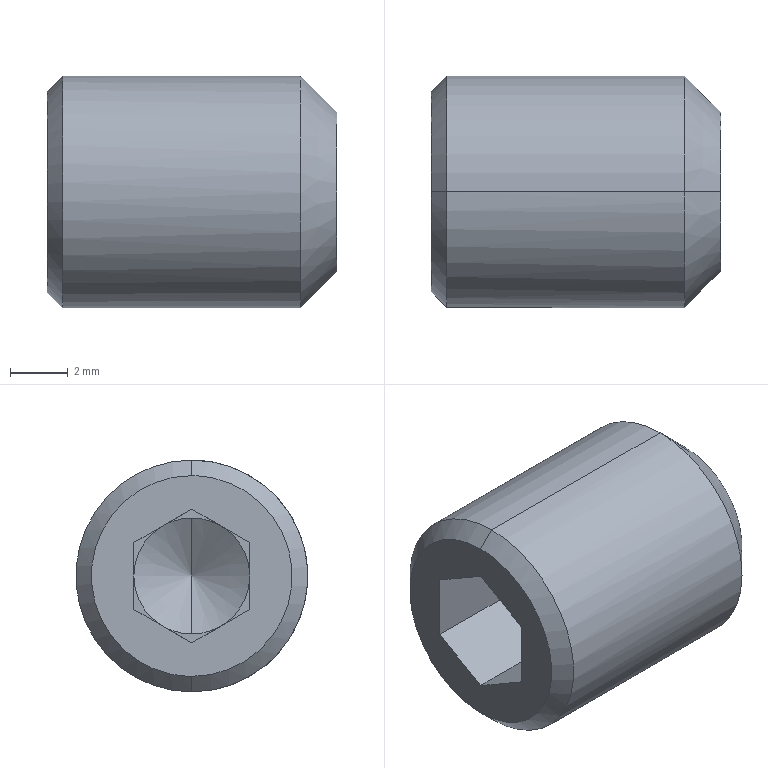Part | STEP file | 103000006174_M8×10 | 1 solid | 22 faces | box 10 x 8 x 8 mm | volume 407.497 mm3 | plane 14 | cone 6 | cylinder 2 | commonest cylinder face diameters 8 x2
STEP:
#1=CARTESIAN_POINT('',(6.155,0.,0.));
#2=VERTEX_POINT('',#1);
#3=CARTESIAN_POINT('',(5.,0.,2.));
#4=VERTEX_POINT('',#3);
#5=CARTESIAN_POINT('',(-250493.845,0.,433878.727));
#6=DIRECTION('',(-0.5,0.,0.866));
#7=VECTOR('',#6,1.);
#8=LINE('',#5,#7);
#9=EDGE_CURVE('',#2,#4,#8,.T.);
#10=ORIENTED_EDGE('',*,*,#9,.F.);
#11=CARTESIAN_POINT('',(5.,0.,-2.));
#12=VERTEX_POINT('',#11);
#13=CARTESIAN_POINT('',(-250493.845,0.,-433878.727));
#14=DIRECTION('',(-0.5,0.,-0.866));
#15=VECTOR('',#14,1.);
#16=LINE('',#13,#15);
#17=EDGE_CURVE('',#2,#12,#16,.T.);
#18=ORIENTED_EDGE('',*,*,#17,.T.);
#19=CARTESIAN_POINT('',(5.,-1.,-1.732));
#20=VERTEX_POINT('',#19);
#21=CARTESIAN_POINT('',(5.,0.,0.));
#22=DIRECTION('',(-1.,0.,0.));
#23=AXIS2_PLACEMENT_3D('',#21,#22,$);
#24=CIRCLE('',#23,2.);
#25=EDGE_CURVE('',#12,#20,#24,.T.);
#26=ORIENTED_EDGE('',*,*,#25,.T.);
#27=CARTESIAN_POINT('',(5.,-2.,0.));
#28=VERTEX_POINT('',#27);
#29=CARTESIAN_POINT('',(5.,0.,0.));
#30=DIRECTION('',(-1.,0.,0.));
#31=AXIS2_PLACEMENT_3D('',#29,#30,$);
#32=CIRCLE('',#31,2.);
#33=EDGE_CURVE('',#20,#28,#32,.T.);
#34=ORIENTED_EDGE('',*,*,#33,.T.);
#35=CARTESIAN_POINT('',(5.,-1.,1.732));
#36=VERTEX_POINT('',#35);
#37=CARTESIAN_POINT('',(5.,0.,0.));
#38=DIRECTION('',(-1.,0.,0.));
#39=AXIS2_PLACEMENT_3D('',#37,#38,$);
#40=CIRCLE('',#39,2.);
#41=EDGE_CURVE('',#28,#36,#40,.T.);
#42=ORIENTED_EDGE('',*,*,#41,.T.);
#43=CARTESIAN_POINT('',(5.,0.,0.));
#44=DIRECTION('',(-1.,0.,0.));
#45=AXIS2_PLACEMENT_3D('',#43,#44,$);
#46=CIRCLE('',#45,2.);
#47=EDGE_CURVE('',#36,#4,#46,.T.);
#48=ORIENTED_EDGE('',*,*,#47,.T.);
#49=EDGE_LOOP('',(#10,#18,#26,#34,#42,#48));
#50=FACE_OUTER_BOUND('',#49,.T.);
#51=CARTESIAN_POINT('',(-993.845,0.,0.));
#52=DIRECTION('',(-1.,0.,0.));
#53=DIRECTION('',(0.,0.,-1.));
#54=AXIS2_PLACEMENT_3D('',#51,#52,#53);
#55=CONICAL_SURFACE('',#54,1732.051,1.047);
#56=ADVANCED_FACE('',(#50),#55,.F.);
#57=ORIENTED_EDGE('',*,*,#17,.F.);
#58=ORIENTED_EDGE('',*,*,#9,.T.);
#59=CARTESIAN_POINT('',(5.,1.,1.732));
#60=VERTEX_POINT('',#59);
#61=CARTESIAN_POINT('',(5.,0.,0.));
#62=DIRECTION('',(-1.,0.,0.));
#63=AXIS2_PLACEMENT_3D('',#61,#62,$);
#64=CIRCLE('',#63,2.);
#65=EDGE_CURVE('',#4,#60,#64,.T.);
#66=ORIENTED_EDGE('',*,*,#65,.T.);
#67=CARTESIAN_POINT('',(5.,2.,0.));
#68=VERTEX_POINT('',#67);
#69=CARTESIAN_POINT('',(5.,0.,0.));
#70=DIRECTION('',(-1.,0.,0.));
#71=AXIS2_PLACEMENT_3D('',#69,#70,$);
#72=CIRCLE('',#71,2.);
#73=EDGE_CURVE('',#60,#68,#72,.T.);
#74=ORIENTED_EDGE('',*,*,#73,.T.);
#75=CARTESIAN_POINT('',(5.,1.,-1.732));
#76=VERTEX_POINT('',#75);
#77=CARTESIAN_POINT('',(5.,0.,0.));
#78=DIRECTION('',(-1.,0.,0.));
#79=AXIS2_PLACEMENT_3D('',#77,#78,$);
#80=CIRCLE('',#79,2.);
#81=EDGE_CURVE('',#68,#76,#80,.T.);
#82=ORIENTED_EDGE('',*,*,#81,.T.);
#83=CARTESIAN_POINT('',(5.,0.,0.));
#84=DIRECTION('',(-1.,0.,0.));
#85=AXIS2_PLACEMENT_3D('',#83,#84,$);
#86=CIRCLE('',#85,2.);
#87=EDGE_CURVE('',#76,#12,#86,.T.);
#88=ORIENTED_EDGE('',*,*,#87,.T.);
#89=EDGE_LOOP('',(#57,#58,#66,#74,#82,#88));
#90=FACE_OUTER_BOUND('',#89,.T.);
#91=CARTESIAN_POINT('',(-993.845,0.,0.));
#92=DIRECTION('',(-1.,0.,0.));
#93=DIRECTION('',(0.,0.,1.));
#94=AXIS2_PLACEMENT_3D('',#91,#92,#93);
#95=CONICAL_SURFACE('',#94,1732.051,1.047);
#96=ADVANCED_FACE('',(#90),#95,.F.);
#97=ORIENTED_EDGE('',*,*,#87,.F.);
#98=CARTESIAN_POINT('',(5.,0.,-2.309));
#99=VERTEX_POINT('',#98);
#100=CARTESIAN_POINT('',(5.,0.5,-2.021));
#101=DIRECTION('',(0.,-0.866,-0.5));
#102=VECTOR('',#101,1.);
#103=LINE('',#100,#102);
#104=EDGE_CURVE('',#76,#99,#103,.T.);
#105=ORIENTED_EDGE('',*,*,#104,.T.);
#106=CARTESIAN_POINT('',(5.,-0.5,-2.021));
#107=DIRECTION('',(0.,-0.866,0.5));
#108=VECTOR('',#107,1.);
#109=LINE('',#106,#108);
#110=EDGE_CURVE('',#99,#20,#109,.T.);
#111=ORIENTED_EDGE('',*,*,#110,.T.);
#112=ORIENTED_EDGE('',*,*,#25,.F.);
#113=EDGE_LOOP('',(#97,#105,#111,#112));
#114=FACE_OUTER_BOUND('',#113,.T.);
#115=CARTESIAN_POINT('',(5.,0.,-2.309));
#116=DIRECTION('',(1.,0.,0.));
#117=DIRECTION('',(0.,0.,-1.));
#118=AXIS2_PLACEMENT_3D('',#115,#116,#117);
#119=PLANE('',#118);
#120=ADVANCED_FACE('',(#114),#119,.F.);
#121=ORIENTED_EDGE('',*,*,#33,.F.);
#122=CARTESIAN_POINT('',(5.,-2.,-1.155));
#123=VERTEX_POINT('',#122);
#124=CARTESIAN_POINT('',(5.,-1.5,-1.443));
#125=DIRECTION('',(0.,-0.866,0.5));
#126=VECTOR('',#125,1.);
#127=LINE('',#124,#126);
#128=EDGE_CURVE('',#20,#123,#127,.T.);
#129=ORIENTED_EDGE('',*,*,#128,.T.);
#130=CARTESIAN_POINT('',(5.,-2.,-0.5774));
#131=DIRECTION('',(0.,0.,1.));
#132=VECTOR('',#131,1.);
#133=LINE('',#130,#132);
#134=EDGE_CURVE('',#123,#28,#133,.T.);
#135=ORIENTED_EDGE('',*,*,#134,.T.);
#136=EDGE_LOOP('',(#121,#129,#135));
#137=FACE_OUTER_BOUND('',#136,.T.);
#138=CARTESIAN_POINT('',(5.,0.,-2.309));
#139=DIRECTION('',(1.,0.,0.));
#140=DIRECTION('',(0.,0.,-1.));
#141=AXIS2_PLACEMENT_3D('',#138,#139,#140);
#142=PLANE('',#141);
#143=ADVANCED_FACE('',(#137),#142,.F.);
#144=ORIENTED_EDGE('',*,*,#41,.F.);
#145=CARTESIAN_POINT('',(5.,-2.,1.155));
#146=VERTEX_POINT('',#145);
#147=CARTESIAN_POINT('',(5.,-2.,0.5774));
#148=DIRECTION('',(0.,0.,1.));
#149=VECTOR('',#148,1.);
#150=LINE('',#147,#149);
#151=EDGE_CURVE('',#28,#146,#150,.T.);
#152=ORIENTED_EDGE('',*,*,#151,.T.);
#153=CARTESIAN_POINT('',(5.,-1.5,1.443));
#154=DIRECTION('',(0.,0.866,0.5));
#155=VECTOR('',#154,1.);
#156=LINE('',#153,#155);
#157=EDGE_CURVE('',#146,#36,#156,.T.);
#158=ORIENTED_EDGE('',*,*,#157,.T.);
#159=EDGE_LOOP('',(#144,#152,#158));
#160=FACE_OUTER_BOUND('',#159,.T.);
#161=CARTESIAN_POINT('',(5.,0.,-2.309));
#162=DIRECTION('',(1.,0.,0.));
#163=DIRECTION('',(0.,0.,-1.));
#164=AXIS2_PLACEMENT_3D('',#161,#162,#163);
#165=PLANE('',#164);
#166=ADVANCED_FACE('',(#160),#165,.F.);
#167=ORIENTED_EDGE('',*,*,#47,.F.);
#168=CARTESIAN_POINT('',(5.,0.,2.309));
#169=VERTEX_POINT('',#168);
#170=CARTESIAN_POINT('',(5.,-0.5,2.021));
#171=DIRECTION('',(0.,0.866,0.5));
#172=VECTOR('',#171,1.);
#173=LINE('',#170,#172);
#174=EDGE_CURVE('',#36,#169,#173,.T.);
#175=ORIENTED_EDGE('',*,*,#174,.T.);
#176=CARTESIAN_POINT('',(5.,0.5,2.021));
#177=DIRECTION('',(0.,0.866,-0.5));
#178=VECTOR('',#177,1.);
#179=LINE('',#176,#178);
#180=EDGE_CURVE('',#169,#60,#179,.T.);
#181=ORIENTED_EDGE('',*,*,#180,.T.);
#182=ORIENTED_EDGE('',*,*,#65,.F.);
#183=EDGE_LOOP('',(#167,#175,#181,#182));
#184=FACE_OUTER_BOUND('',#183,.T.);
#185=CARTESIAN_POINT('',(5.,0.,-2.309));
#186=DIRECTION('',(1.,0.,0.));
#187=DIRECTION('',(0.,0.,-1.));
#188=AXIS2_PLACEMENT_3D('',#185,#186,#187);
#189=PLANE('',#188);
#190=ADVANCED_FACE('',(#184),#189,.F.);
#191=ORIENTED_EDGE('',*,*,#73,.F.);
#192=CARTESIAN_POINT('',(5.,2.,1.155));
#193=VERTEX_POINT('',#192);
#194=CARTESIAN_POINT('',(5.,1.5,1.443));
#195=DIRECTION('',(0.,0.866,-0.5));
#196=VECTOR('',#195,1.);
#197=LINE('',#194,#196);
#198=EDGE_CURVE('',#60,#193,#197,.T.);
#199=ORIENTED_EDGE('',*,*,#198,.T.);
#200=CARTESIAN_POINT('',(5.,2.,0.5774));
#201=DIRECTION('',(0.,0.,-1.));
#202=VECTOR('',#201,1.);
#203=LINE('',#200,#202);
#204=EDGE_CURVE('',#193,#68,#203,.T.);
#205=ORIENTED_EDGE('',*,*,#204,.T.);
#206=EDGE_LOOP('',(#191,#199,#205));
#207=FACE_OUTER_BOUND('',#206,.T.);
#208=CARTESIAN_POINT('',(5.,0.,-2.309));
#209=DIRECTION('',(1.,0.,0.));
#210=DIRECTION('',(0.,0.,-1.));
#211=AXIS2_PLACEMENT_3D('',#208,#209,#210);
#212=PLANE('',#211);
#213=ADVANCED_FACE('',(#207),#212,.F.);
#214=ORIENTED_EDGE('',*,*,#81,.F.);
#215=CARTESIAN_POINT('',(5.,2.,-1.155));
#216=VERTEX_POINT('',#215);
#217=CARTESIAN_POINT('',(5.,2.,-0.5774));
#218=DIRECTION('',(0.,0.,-1.));
#219=VECTOR('',#218,1.);
#220=LINE('',#217,#219);
#221=EDGE_CURVE('',#68,#216,#220,.T.);
#222=ORIENTED_EDGE('',*,*,#221,.T.);
#223=CARTESIAN_POINT('',(5.,1.5,-1.443));
#224=DIRECTION('',(0.,-0.866,-0.5));
#225=VECTOR('',#224,1.);
#226=LINE('',#223,#225);
#227=EDGE_CURVE('',#216,#76,#226,.T.);
#228=ORIENTED_EDGE('',*,*,#227,.T.);
#229=EDGE_LOOP('',(#214,#222,#228));
#230=FACE_OUTER_BOUND('',#229,.T.);
#231=CARTESIAN_POINT('',(5.,0.,-2.309));
#232=DIRECTION('',(1.,0.,0.));
#233=DIRECTION('',(0.,0.,-1.));
#234=AXIS2_PLACEMENT_3D('',#231,#232,#233);
#235=PLANE('',#234);
#236=ADVANCED_FACE('',(#230),#235,.F.);
#237=CARTESIAN_POINT('',(0.,2.,-1.155));
#238=VERTEX_POINT('',#237);
#239=CARTESIAN_POINT('',(0.,0.,-2.309));
#240=VERTEX_POINT('',#239);
#241=CARTESIAN_POINT('',(0.,1.,-1.732));
#242=DIRECTION('',(0.,-0.866,-0.5));
#243=VECTOR('',#242,1.);
#244=LINE('',#241,#243);
#245=EDGE_CURVE('',#238,#240,#244,.T.);
#246=ORIENTED_EDGE('',*,*,#245,.T.);
#247=CARTESIAN_POINT('',(2.5,0.,-2.309));
#248=DIRECTION('',(-1.,0.,0.));
#249=VECTOR('',#248,1.);
#250=LINE('',#247,#249);
#251=EDGE_CURVE('',#99,#240,#250,.T.);
#252=ORIENTED_EDGE('',*,*,#251,.F.);
#253=ORIENTED_EDGE('',*,*,#104,.F.);
#254=ORIENTED_EDGE('',*,*,#227,.F.);
#255=CARTESIAN_POINT('',(2.5,2.,-1.155));
#256=DIRECTION('',(-1.,0.,0.));
#257=VECTOR('',#256,1.);
#258=LINE('',#255,#257);
#259=EDGE_CURVE('',#216,#238,#258,.T.);
#260=ORIENTED_EDGE('',*,*,#259,.T.);
#261=EDGE_LOOP('',(#246,#252,#253,#254,#260));
#262=FACE_OUTER_BOUND('',#261,.T.);
#263=CARTESIAN_POINT('',(5.,2.,-1.155));
#264=DIRECTION('',(0.,0.5,-0.866));
#265=DIRECTION('',(0.,0.866,0.5));
#266=AXIS2_PLACEMENT_3D('',#263,#264,#265);
#267=PLANE('',#266);
#268=ADVANCED_FACE('',(#262),#267,.F.);
#269=CARTESIAN_POINT('',(0.,-2.,-1.155));
#270=VERTEX_POINT('',#269);
#271=CARTESIAN_POINT('',(0.,-1.,-1.732));
#272=DIRECTION('',(0.,-0.866,0.5));
#273=VECTOR('',#272,1.);
#274=LINE('',#271,#273);
#275=EDGE_CURVE('',#240,#270,#274,.T.);
#276=ORIENTED_EDGE('',*,*,#275,.T.);
#277=CARTESIAN_POINT('',(2.5,-2.,-1.155));
#278=DIRECTION('',(-1.,0.,0.));
#279=VECTOR('',#278,1.);
#280=LINE('',#277,#279);
#281=EDGE_CURVE('',#123,#270,#280,.T.);
#282=ORIENTED_EDGE('',*,*,#281,.F.);
#283=ORIENTED_EDGE('',*,*,#128,.F.);
#284=ORIENTED_EDGE('',*,*,#110,.F.);
#285=ORIENTED_EDGE('',*,*,#251,.T.);
#286=EDGE_LOOP('',(#276,#282,#283,#284,#285));
#287=FACE_OUTER_BOUND('',#286,.T.);
#288=CARTESIAN_POINT('',(5.,0.,-2.309));
#289=DIRECTION('',(0.,-0.5,-0.866));
#290=DIRECTION('',(0.,0.866,-0.5));
#291=AXIS2_PLACEMENT_3D('',#288,#289,#290);
#292=PLANE('',#291);
#293=ADVANCED_FACE('',(#287),#292,.F.);
#294=CARTESIAN_POINT('',(0.,-2.,1.155));
#295=VERTEX_POINT('',#294);
#296=CARTESIAN_POINT('',(0.,-2.,0.));
#297=DIRECTION('',(0.,0.,1.));
#298=VECTOR('',#297,1.);
#299=LINE('',#296,#298);
#300=EDGE_CURVE('',#270,#295,#299,.T.);
#301=ORIENTED_EDGE('',*,*,#300,.T.);
#302=CARTESIAN_POINT('',(2.5,-2.,1.155));
#303=DIRECTION('',(-1.,0.,0.));
#304=VECTOR('',#303,1.);
#305=LINE('',#302,#304);
#306=EDGE_CURVE('',#146,#295,#305,.T.);
#307=ORIENTED_EDGE('',*,*,#306,.F.);
#308=ORIENTED_EDGE('',*,*,#151,.F.);
#309=ORIENTED_EDGE('',*,*,#134,.F.);
#310=ORIENTED_EDGE('',*,*,#281,.T.);
#311=EDGE_LOOP('',(#301,#307,#308,#309,#310));
#312=FACE_OUTER_BOUND('',#311,.T.);
#313=CARTESIAN_POINT('',(5.,-2.,-1.155));
#314=DIRECTION('',(0.,-1.,0.));
#315=DIRECTION('',(0.,0.,-1.));
#316=AXIS2_PLACEMENT_3D('',#313,#314,#315);
#317=PLANE('',#316);
#318=ADVANCED_FACE('',(#312),#317,.F.);
#319=CARTESIAN_POINT('',(0.,0.,2.309));
#320=VERTEX_POINT('',#319);
#321=CARTESIAN_POINT('',(0.,-1.,1.732));
#322=DIRECTION('',(0.,0.866,0.5));
#323=VECTOR('',#322,1.);
#324=LINE('',#321,#323);
#325=EDGE_CURVE('',#295,#320,#324,.T.);
#326=ORIENTED_EDGE('',*,*,#325,.T.);
#327=CARTESIAN_POINT('',(2.5,0.,2.309));
#328=DIRECTION('',(-1.,0.,0.));
#329=VECTOR('',#328,1.);
#330=LINE('',#327,#329);
#331=EDGE_CURVE('',#169,#320,#330,.T.);
#332=ORIENTED_EDGE('',*,*,#331,.F.);
#333=ORIENTED_EDGE('',*,*,#174,.F.);
#334=ORIENTED_EDGE('',*,*,#157,.F.);
#335=ORIENTED_EDGE('',*,*,#306,.T.);
#336=EDGE_LOOP('',(#326,#332,#333,#334,#335));
#337=FACE_OUTER_BOUND('',#336,.T.);
#338=CARTESIAN_POINT('',(5.,-2.,1.155));
#339=DIRECTION('',(0.,-0.5,0.866));
#340=DIRECTION('',(0.,-0.866,-0.5));
#341=AXIS2_PLACEMENT_3D('',#338,#339,#340);
#342=PLANE('',#341);
#343=ADVANCED_FACE('',(#337),#342,.F.);
#344=CARTESIAN_POINT('',(0.,2.,1.155));
#345=VERTEX_POINT('',#344);
#346=CARTESIAN_POINT('',(0.,1.,1.732));
#347=DIRECTION('',(0.,0.866,-0.5));
#348=VECTOR('',#347,1.);
#349=LINE('',#346,#348);
#350=EDGE_CURVE('',#320,#345,#349,.T.);
#351=ORIENTED_EDGE('',*,*,#350,.T.);
#352=CARTESIAN_POINT('',(2.5,2.,1.155));
#353=DIRECTION('',(-1.,0.,0.));
#354=VECTOR('',#353,1.);
#355=LINE('',#352,#354);
#356=EDGE_CURVE('',#193,#345,#355,.T.);
#357=ORIENTED_EDGE('',*,*,#356,.F.);
#358=ORIENTED_EDGE('',*,*,#198,.F.);
#359=ORIENTED_EDGE('',*,*,#180,.F.);
#360=ORIENTED_EDGE('',*,*,#331,.T.);
#361=EDGE_LOOP('',(#351,#357,#358,#359,#360));
#362=FACE_OUTER_BOUND('',#361,.T.);
#363=CARTESIAN_POINT('',(5.,0.,2.309));
#364=DIRECTION('',(0.,0.5,0.866));
#365=DIRECTION('',(0.,-0.866,0.5));
#366=AXIS2_PLACEMENT_3D('',#363,#364,#365);
#367=PLANE('',#366);
#368=ADVANCED_FACE('',(#362),#367,.F.);
#369=CARTESIAN_POINT('',(0.,2.,0.));
#370=DIRECTION('',(0.,0.,-1.));
#371=VECTOR('',#370,1.);
#372=LINE('',#369,#371);
#373=EDGE_CURVE('',#345,#238,#372,.T.);
#374=ORIENTED_EDGE('',*,*,#373,.T.);
#375=ORIENTED_EDGE('',*,*,#259,.F.);
#376=ORIENTED_EDGE('',*,*,#221,.F.);
#377=ORIENTED_EDGE('',*,*,#204,.F.);
#378=ORIENTED_EDGE('',*,*,#356,.T.);
#379=EDGE_LOOP('',(#374,#375,#376,#377,#378));
#380=FACE_OUTER_BOUND('',#379,.T.);
#381=CARTESIAN_POINT('',(5.,2.,1.155));
#382=DIRECTION('',(0.,1.,0.));
#383=DIRECTION('',(0.,0.,1.));
#384=AXIS2_PLACEMENT_3D('',#381,#382,#383);
#385=PLANE('',#384);
#386=ADVANCED_FACE('',(#380),#385,.F.);
#387=CARTESIAN_POINT('',(0.,0.,-3.464));
#388=VERTEX_POINT('',#387);
#389=CARTESIAN_POINT('',(0.,0.,3.464));
#390=VERTEX_POINT('',#389);
#391=CARTESIAN_POINT('',(0.,0.,-3.464));
#392=CARTESIAN_POINT('',(0.,-0.3647,-3.464));
#393=CARTESIAN_POINT('',(0.,-0.7294,-3.416));
#394=CARTESIAN_POINT('',(0.,-1.086,-3.32));
#395=CARTESIAN_POINT('',(0.,-1.765,-3.036));
#396=CARTESIAN_POINT('',(0.,-2.347,-2.587));
#397=CARTESIAN_POINT('',(0.,-2.607,-2.325));
#398=CARTESIAN_POINT('',(0.,-3.051,-1.739));
#399=CARTESIAN_POINT('',(0.,-3.329,-1.057));
#400=CARTESIAN_POINT('',(0.,-3.422,-0.7003));
#401=CARTESIAN_POINT('',(0.,-3.512,0.02991));
#402=CARTESIAN_POINT('',(0.,-3.41,0.7585));
#403=CARTESIAN_POINT('',(0.,-3.311,1.114));
#404=CARTESIAN_POINT('',(0.,-3.021,1.79));
#405=CARTESIAN_POINT('',(0.,-2.567,2.369));
#406=CARTESIAN_POINT('',(0.,-2.303,2.627));
#407=CARTESIAN_POINT('',(0.,-1.722,3.059));
#408=CARTESIAN_POINT('',(0.,-1.051,3.329));
#409=CARTESIAN_POINT('',(0.,-0.7058,3.419));
#410=CARTESIAN_POINT('',(0.,-0.3529,3.464));
#411=CARTESIAN_POINT('',(0.,0.,3.464));
#412=B_SPLINE_CURVE_WITH_KNOTS('',5,(#391,#392,#393,#394,#395,#396,#397,#398,#399,#400,#401,#402,#403,#404,#405,#406,#407,#408,#409,#410,#411),.UNSPECIFIED.,.F.,.U.,(6,3,3,3,3,3,6),(0.,2.579,5.158,7.737,10.316,12.894,15.39),.UNSPECIFIED.);
#413=EDGE_CURVE('',#388,#390,#412,.T.);
#414=ORIENTED_EDGE('',*,*,#413,.T.);
#415=CARTESIAN_POINT('',(0.,0.,3.464));
#416=CARTESIAN_POINT('',(0.,0.3647,3.464));
#417=CARTESIAN_POINT('',(0.,0.7294,3.416));
#418=CARTESIAN_POINT('',(0.,1.086,3.32));
#419=CARTESIAN_POINT('',(0.,1.765,3.036));
#420=CARTESIAN_POINT('',(0.,2.347,2.587));
#421=CARTESIAN_POINT('',(0.,2.607,2.325));
#422=CARTESIAN_POINT('',(0.,3.051,1.739));
#423=CARTESIAN_POINT('',(0.,3.329,1.057));
#424=CARTESIAN_POINT('',(0.,3.422,0.7003));
#425=CARTESIAN_POINT('',(0.,3.512,-0.02991));
#426=CARTESIAN_POINT('',(0.,3.41,-0.7585));
#427=CARTESIAN_POINT('',(0.,3.311,-1.114));
#428=CARTESIAN_POINT('',(0.,3.021,-1.79));
#429=CARTESIAN_POINT('',(0.,2.567,-2.369));
#430=CARTESIAN_POINT('',(0.,2.303,-2.627));
#431=CARTESIAN_POINT('',(0.,1.722,-3.059));
#432=CARTESIAN_POINT('',(0.,1.051,-3.329));
#433=CARTESIAN_POINT('',(0.,0.7058,-3.419));
#434=CARTESIAN_POINT('',(0.,0.3529,-3.464));
#435=CARTESIAN_POINT('',(0.,0.,-3.464));
#436=B_SPLINE_CURVE_WITH_KNOTS('',5,(#415,#416,#417,#418,#419,#420,#421,#422,#423,#424,#425,#426,#427,#428,#429,#430,#431,#432,#433,#434,#435),.UNSPECIFIED.,.F.,.U.,(6,3,3,3,3,3,6),(0.,2.579,5.158,7.737,10.316,12.894,15.39),.UNSPECIFIED.);
#437=EDGE_CURVE('',#390,#388,#436,.T.);
#438=ORIENTED_EDGE('',*,*,#437,.T.);
#439=EDGE_LOOP('',(#414,#438));
#440=FACE_OUTER_BOUND('',#439,.T.);
#441=ORIENTED_EDGE('',*,*,#300,.F.);
#442=ORIENTED_EDGE('',*,*,#275,.F.);
#443=ORIENTED_EDGE('',*,*,#245,.F.);
#444=ORIENTED_EDGE('',*,*,#373,.F.);
#445=ORIENTED_EDGE('',*,*,#350,.F.);
#446=ORIENTED_EDGE('',*,*,#325,.F.);
#447=EDGE_LOOP('',(#441,#442,#443,#444,#445,#446));
#448=FACE_BOUND('',#447,.T.);
#449=CARTESIAN_POINT('',(0.,3.464,0.));
#450=DIRECTION('',(1.,0.,0.));
#451=DIRECTION('',(0.,0.,-1.));
#452=AXIS2_PLACEMENT_3D('',#449,#450,#451);
#453=PLANE('',#452);
#454=ADVANCED_FACE('',(#440,#448),#453,.F.);
#455=CARTESIAN_POINT('',(0.536,0.,4.));
#456=VERTEX_POINT('',#455);
#457=CARTESIAN_POINT('',(353551.927,0.,353555.391));
#458=DIRECTION('',(0.7071,0.,0.7071));
#459=VECTOR('',#458,1.);
#460=LINE('',#457,#459);
#461=EDGE_CURVE('',#390,#456,#460,.T.);
#462=ORIENTED_EDGE('',*,*,#461,.F.);
#463=ORIENTED_EDGE('',*,*,#413,.F.);
#464=CARTESIAN_POINT('',(0.536,0.,-4.));
#465=VERTEX_POINT('',#464);
#466=CARTESIAN_POINT('',(353551.927,0.,-353555.391));
#467=DIRECTION('',(0.7071,0.,-0.7071));
#468=VECTOR('',#467,1.);
#469=LINE('',#466,#468);
#470=EDGE_CURVE('',#388,#465,#469,.T.);
#471=ORIENTED_EDGE('',*,*,#470,.T.);
#472=CARTESIAN_POINT('',(0.536,0.,0.));
#473=DIRECTION('',(1.,0.,0.));
#474=AXIS2_PLACEMENT_3D('',#472,#473,$);
#475=CIRCLE('',#474,4.);
#476=EDGE_CURVE('',#465,#456,#475,.F.);
#477=ORIENTED_EDGE('',*,*,#476,.T.);
#478=EDGE_LOOP('',(#462,#463,#471,#477));
#479=FACE_OUTER_BOUND('',#478,.T.);
#480=CARTESIAN_POINT('',(0.536,0.,0.));
#481=DIRECTION('',(1.,0.,0.));
#482=DIRECTION('',(0.,0.,1.));
#483=AXIS2_PLACEMENT_3D('',#480,#481,#482);
#484=CONICAL_SURFACE('',#483,4.,0.7854);
#485=ADVANCED_FACE('',(#479),#484,.T.);
#486=ORIENTED_EDGE('',*,*,#437,.F.);
#487=ORIENTED_EDGE('',*,*,#461,.T.);
#488=CARTESIAN_POINT('',(0.536,0.,0.));
#489=DIRECTION('',(1.,0.,0.));
#490=AXIS2_PLACEMENT_3D('',#488,#489,$);
#491=CIRCLE('',#490,4.);
#492=EDGE_CURVE('',#456,#465,#491,.F.);
#493=ORIENTED_EDGE('',*,*,#492,.T.);
#494=ORIENTED_EDGE('',*,*,#470,.F.);
#495=EDGE_LOOP('',(#486,#487,#493,#494));
#496=FACE_OUTER_BOUND('',#495,.T.);
#497=CARTESIAN_POINT('',(0.536,0.,0.));
#498=DIRECTION('',(1.,0.,0.));
#499=DIRECTION('',(0.,0.,-1.));
#500=AXIS2_PLACEMENT_3D('',#497,#498,#499);
#501=CONICAL_SURFACE('',#500,4.,0.7854);
#502=ADVANCED_FACE('',(#496),#501,.T.);
#503=CARTESIAN_POINT('',(8.75,0.,-4.));
#504=VERTEX_POINT('',#503);
#505=CARTESIAN_POINT('',(-0.2778,0.,-4.));
#506=DIRECTION('',(-1.,0.,0.));
#507=VECTOR('',#506,1.);
#508=LINE('',#505,#507);
#509=EDGE_CURVE('',#504,#465,#508,.T.);
#510=ORIENTED_EDGE('',*,*,#509,.F.);
#511=CARTESIAN_POINT('',(8.75,0.,4.));
#512=VERTEX_POINT('',#511);
#513=CARTESIAN_POINT('',(8.75,0.,-4.));
#514=CARTESIAN_POINT('',(8.75,-0.6283,-4.));
#515=CARTESIAN_POINT('',(8.75,-1.257,-3.877));
#516=CARTESIAN_POINT('',(8.75,-1.853,-3.63));
#517=CARTESIAN_POINT('',(8.75,-2.916,-2.916));
#518=CARTESIAN_POINT('',(8.75,-3.63,-1.853));
#519=CARTESIAN_POINT('',(8.75,-3.877,-1.257));
#520=CARTESIAN_POINT('',(8.75,-4.123,0.));
#521=CARTESIAN_POINT('',(8.75,-3.877,1.257));
#522=CARTESIAN_POINT('',(8.75,-3.63,1.853));
#523=CARTESIAN_POINT('',(8.75,-2.916,2.916));
#524=CARTESIAN_POINT('',(8.75,-1.853,3.63));
#525=CARTESIAN_POINT('',(8.75,-1.257,3.877));
#526=CARTESIAN_POINT('',(8.75,-0.6283,4.));
#527=CARTESIAN_POINT('',(8.75,0.,4.));
#528=B_SPLINE_CURVE_WITH_KNOTS('',5,(#513,#514,#515,#516,#517,#518,#519,#520,#521,#522,#523,#524,#525,#526,#527),.UNSPECIFIED.,.F.,.U.,(6,3,3,3,6),(-6.283,-3.142,0.,3.142,6.283),.UNSPECIFIED.);
#529=EDGE_CURVE('',#504,#512,#528,.T.);
#530=ORIENTED_EDGE('',*,*,#529,.T.);
#531=CARTESIAN_POINT('',(-0.2778,0.,4.));
#532=DIRECTION('',(-1.,0.,0.));
#533=VECTOR('',#532,1.);
#534=LINE('',#531,#533);
#535=EDGE_CURVE('',#512,#456,#534,.T.);
#536=ORIENTED_EDGE('',*,*,#535,.T.);
#537=ORIENTED_EDGE('',*,*,#476,.F.);
#538=EDGE_LOOP('',(#510,#530,#536,#537));
#539=FACE_OUTER_BOUND('',#538,.T.);
#540=CARTESIAN_POINT('',(-0.2778,0.,0.));
#541=DIRECTION('',(-1.,0.,0.));
#542=DIRECTION('',(0.,0.,-1.));
#543=AXIS2_PLACEMENT_3D('',#540,#541,#542);
#544=CYLINDRICAL_SURFACE('',#543,4.);
#545=ADVANCED_FACE('',(#539),#544,.T.);
#546=CARTESIAN_POINT('',(8.75,0.,0.));
#547=DIRECTION('',(-1.,0.,0.));
#548=AXIS2_PLACEMENT_3D('',#546,#547,$);
#549=CIRCLE('',#548,4.);
#550=EDGE_CURVE('',#512,#504,#549,.T.);
#551=ORIENTED_EDGE('',*,*,#550,.T.);
#552=ORIENTED_EDGE('',*,*,#509,.T.);
#553=ORIENTED_EDGE('',*,*,#492,.F.);
#554=ORIENTED_EDGE('',*,*,#535,.F.);
#555=EDGE_LOOP('',(#551,#552,#553,#554));
#556=FACE_OUTER_BOUND('',#555,.T.);
#557=CARTESIAN_POINT('',(-0.2778,0.,0.));
#558=DIRECTION('',(-1.,0.,0.));
#559=DIRECTION('',(0.,0.,1.));
#560=AXIS2_PLACEMENT_3D('',#557,#558,#559);
#561=CYLINDRICAL_SURFACE('',#560,4.);
#562=ADVANCED_FACE('',(#556),#561,.T.);
#563=CARTESIAN_POINT('',(10.,0.,-2.75));
#564=VERTEX_POINT('',#563);
#565=CARTESIAN_POINT('',(-353542.016,0.,-353554.766));
#566=DIRECTION('',(-0.7071,0.,-0.7071));
#567=VECTOR('',#566,1.);
#568=LINE('',#565,#567);
#569=EDGE_CURVE('',#564,#504,#568,.T.);
#570=ORIENTED_EDGE('',*,*,#569,.F.);
#571=CARTESIAN_POINT('',(10.,0.,2.75));
#572=VERTEX_POINT('',#571);
#573=CARTESIAN_POINT('',(10.,0.,0.));
#574=DIRECTION('',(-1.,0.,0.));
#575=AXIS2_PLACEMENT_3D('',#573,#574,$);
#576=CIRCLE('',#575,2.75);
#577=EDGE_CURVE('',#564,#572,#576,.T.);
#578=ORIENTED_EDGE('',*,*,#577,.T.);
#579=CARTESIAN_POINT('',(-353542.016,0.,353554.766));
#580=DIRECTION('',(-0.7071,0.,0.7071));
#581=VECTOR('',#580,1.);
#582=LINE('',#579,#581);
#583=EDGE_CURVE('',#572,#512,#582,.T.);
#584=ORIENTED_EDGE('',*,*,#583,.T.);
#585=ORIENTED_EDGE('',*,*,#529,.F.);
#586=EDGE_LOOP('',(#570,#578,#584,#585));
#587=FACE_OUTER_BOUND('',#586,.T.);
#588=CARTESIAN_POINT('',(10.,0.,0.));
#589=DIRECTION('',(-1.,0.,0.));
#590=DIRECTION('',(0.,0.,-1.));
#591=AXIS2_PLACEMENT_3D('',#588,#589,#590);
#592=CONICAL_SURFACE('',#591,2.75,0.7854);
#593=ADVANCED_FACE('',(#587),#592,.T.);
#594=CARTESIAN_POINT('',(10.,0.,0.));
#595=DIRECTION('',(-1.,0.,0.));
#596=AXIS2_PLACEMENT_3D('',#594,#595,$);
#597=CIRCLE('',#596,2.75);
#598=EDGE_CURVE('',#572,#564,#597,.T.);
#599=ORIENTED_EDGE('',*,*,#598,.T.);
#600=ORIENTED_EDGE('',*,*,#569,.T.);
#601=ORIENTED_EDGE('',*,*,#550,.F.);
#602=ORIENTED_EDGE('',*,*,#583,.F.);
#603=EDGE_LOOP('',(#599,#600,#601,#602));
#604=FACE_OUTER_BOUND('',#603,.T.);
#605=CARTESIAN_POINT('',(10.,0.,0.));
#606=DIRECTION('',(-1.,0.,0.));
#607=DIRECTION('',(0.,0.,1.));
#608=AXIS2_PLACEMENT_3D('',#605,#606,#607);
#609=CONICAL_SURFACE('',#608,2.75,0.7854);
#610=ADVANCED_FACE('',(#604),#609,.T.);
#611=ORIENTED_EDGE('',*,*,#598,.F.);
#612=ORIENTED_EDGE('',*,*,#577,.F.);
#613=EDGE_LOOP('',(#611,#612));
#614=FACE_OUTER_BOUND('',#613,.T.);
#615=CARTESIAN_POINT('',(10.,0.,0.));
#616=DIRECTION('',(-1.,0.,0.));
#617=DIRECTION('',(0.,0.,1.));
#618=AXIS2_PLACEMENT_3D('',#615,#616,#617);
#619=PLANE('',#618);
#620=ADVANCED_FACE('',(#614),#619,.F.);
#621=CLOSED_SHELL('',(#56,#96,#120,#143,#166,#190,#213,#236,#268,#293,#318,#343,#368,#386,#454,#485,#502,#545,#562,#593,#610,#620));
#622=MANIFOLD_SOLID_BREP('',#621);
#623=(LENGTH_UNIT()NAMED_UNIT(*)SI_UNIT(.MILLI.,.METRE.));
#624=UNCERTAINTY_MEASURE_WITH_UNIT(LENGTH_MEASURE(0.005),#623,'','');
#625=(NAMED_UNIT(*)PLANE_ANGLE_UNIT()SI_UNIT($,.RADIAN.));
#626=(NAMED_UNIT(*)SI_UNIT($,.STERADIAN.)SOLID_ANGLE_UNIT());
#627=(GEOMETRIC_REPRESENTATION_CONTEXT(3)GLOBAL_UNCERTAINTY_ASSIGNED_CONTEXT((#624))GLOBAL_UNIT_ASSIGNED_CONTEXT((#623,#625,#626))REPRESENTATION_CONTEXT('',''));
#628=ADVANCED_BREP_SHAPE_REPRESENTATION('',(#622),#627);